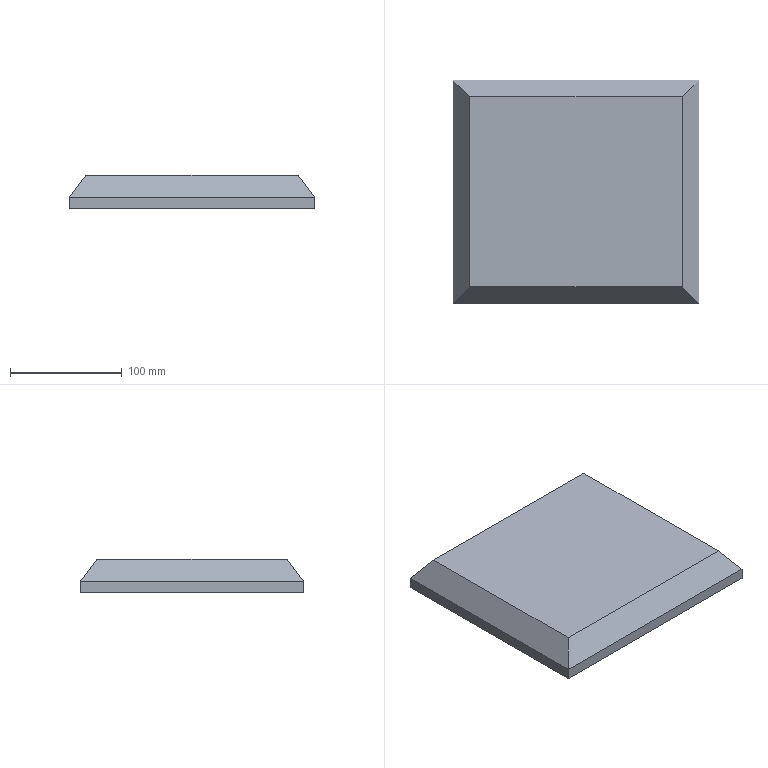Part | SolidWorks | features ICE 1, NetBlend 1 | 1 solid | 10 faces | box 220 x 200 x 30 mm | volume 1200000 mm3 | plane 10
STEP:
#1=CARTESIAN_POINT('',(15.,185.,20.));
#2=VERTEX_POINT('',#1);
#3=CARTESIAN_POINT('',(205.,185.,20.));
#4=VERTEX_POINT('',#3);
#5=CARTESIAN_POINT('',(110.,185.,20.));
#6=DIRECTION('',(1.,0.,0.));
#7=VECTOR('',#6,1000.);
#8=LINE('',#5,#7);
#9=EDGE_CURVE('',#2,#4,#8,.T.);
#10=ORIENTED_EDGE('',*,*,#9,.T.);
#11=CARTESIAN_POINT('',(220.,200.,0.));
#12=VERTEX_POINT('',#11);
#13=CARTESIAN_POINT('',(212.5,192.5,10.));
#14=DIRECTION('',(0.5145,0.5145,-0.686));
#15=VECTOR('',#14,1000.);
#16=LINE('',#13,#15);
#17=EDGE_CURVE('',#4,#12,#16,.T.);
#18=ORIENTED_EDGE('',*,*,#17,.T.);
#19=CARTESIAN_POINT('',(0.,200.,0.));
#20=VERTEX_POINT('',#19);
#21=CARTESIAN_POINT('',(110.,200.,0.));
#22=DIRECTION('',(1.,0.,0.));
#23=VECTOR('',#22,1000.);
#24=LINE('',#21,#23);
#25=EDGE_CURVE('',#20,#12,#24,.T.);
#26=ORIENTED_EDGE('',*,*,#25,.F.);
#27=CARTESIAN_POINT('',(7.5,192.5,10.));
#28=DIRECTION('',(-0.5145,0.5145,-0.686));
#29=VECTOR('',#28,1000.);
#30=LINE('',#27,#29);
#31=EDGE_CURVE('',#2,#20,#30,.T.);
#32=ORIENTED_EDGE('',*,*,#31,.F.);
#33=EDGE_LOOP('',(#10,#18,#26,#32));
#34=FACE_OUTER_BOUND('',#33,.T.);
#35=CARTESIAN_POINT('',(15.,185.,20.));
#36=DIRECTION('',(0.,0.8,0.6));
#37=DIRECTION('',(1.,0.,0.));
#38=AXIS2_PLACEMENT_3D('',#35,#36,#37);
#39=PLANE('',#38);
#40=ADVANCED_FACE('',(#34),#39,.T.);
#41=CARTESIAN_POINT('',(205.,15.,20.));
#42=VERTEX_POINT('',#41);
#43=CARTESIAN_POINT('',(205.,100.,20.));
#44=DIRECTION('',(0.,-1.,0.));
#45=VECTOR('',#44,1000.);
#46=LINE('',#43,#45);
#47=EDGE_CURVE('',#4,#42,#46,.T.);
#48=ORIENTED_EDGE('',*,*,#47,.T.);
#49=CARTESIAN_POINT('',(220.,0.,0.));
#50=VERTEX_POINT('',#49);
#51=CARTESIAN_POINT('',(212.5,7.5,10.));
#52=DIRECTION('',(0.5145,-0.5145,-0.686));
#53=VECTOR('',#52,1000.);
#54=LINE('',#51,#53);
#55=EDGE_CURVE('',#42,#50,#54,.T.);
#56=ORIENTED_EDGE('',*,*,#55,.T.);
#57=CARTESIAN_POINT('',(220.,100.,0.));
#58=DIRECTION('',(0.,-1.,0.));
#59=VECTOR('',#58,1000.);
#60=LINE('',#57,#59);
#61=EDGE_CURVE('',#12,#50,#60,.T.);
#62=ORIENTED_EDGE('',*,*,#61,.F.);
#63=ORIENTED_EDGE('',*,*,#17,.F.);
#64=EDGE_LOOP('',(#48,#56,#62,#63));
#65=FACE_OUTER_BOUND('',#64,.T.);
#66=CARTESIAN_POINT('',(205.,185.,20.));
#67=DIRECTION('',(0.8,0.,0.6));
#68=DIRECTION('',(0.,-1.,0.));
#69=AXIS2_PLACEMENT_3D('',#66,#67,#68);
#70=PLANE('',#69);
#71=ADVANCED_FACE('',(#65),#70,.T.);
#72=CARTESIAN_POINT('',(15.,15.,20.));
#73=VERTEX_POINT('',#72);
#74=CARTESIAN_POINT('',(110.,15.,20.));
#75=DIRECTION('',(-1.,0.,0.));
#76=VECTOR('',#75,1000.);
#77=LINE('',#74,#76);
#78=EDGE_CURVE('',#42,#73,#77,.T.);
#79=ORIENTED_EDGE('',*,*,#78,.T.);
#80=CARTESIAN_POINT('',(0.,0.,0.));
#81=VERTEX_POINT('',#80);
#82=CARTESIAN_POINT('',(7.5,7.5,10.));
#83=DIRECTION('',(-0.5145,-0.5145,-0.686));
#84=VECTOR('',#83,1000.);
#85=LINE('',#82,#84);
#86=EDGE_CURVE('',#73,#81,#85,.T.);
#87=ORIENTED_EDGE('',*,*,#86,.T.);
#88=CARTESIAN_POINT('',(110.,0.,0.));
#89=DIRECTION('',(-1.,0.,0.));
#90=VECTOR('',#89,1000.);
#91=LINE('',#88,#90);
#92=EDGE_CURVE('',#50,#81,#91,.T.);
#93=ORIENTED_EDGE('',*,*,#92,.F.);
#94=ORIENTED_EDGE('',*,*,#55,.F.);
#95=EDGE_LOOP('',(#79,#87,#93,#94));
#96=FACE_OUTER_BOUND('',#95,.T.);
#97=CARTESIAN_POINT('',(205.,15.,20.));
#98=DIRECTION('',(0.,-0.8,0.6));
#99=DIRECTION('',(-1.,0.,0.));
#100=AXIS2_PLACEMENT_3D('',#97,#98,#99);
#101=PLANE('',#100);
#102=ADVANCED_FACE('',(#96),#101,.T.);
#103=CARTESIAN_POINT('',(15.,100.,20.));
#104=DIRECTION('',(0.,1.,0.));
#105=VECTOR('',#104,1000.);
#106=LINE('',#103,#105);
#107=EDGE_CURVE('',#73,#2,#106,.T.);
#108=ORIENTED_EDGE('',*,*,#107,.T.);
#109=ORIENTED_EDGE('',*,*,#31,.T.);
#110=CARTESIAN_POINT('',(0.,100.,0.));
#111=DIRECTION('',(0.,1.,0.));
#112=VECTOR('',#111,1000.);
#113=LINE('',#110,#112);
#114=EDGE_CURVE('',#81,#20,#113,.T.);
#115=ORIENTED_EDGE('',*,*,#114,.F.);
#116=ORIENTED_EDGE('',*,*,#86,.F.);
#117=EDGE_LOOP('',(#108,#109,#115,#116));
#118=FACE_OUTER_BOUND('',#117,.T.);
#119=CARTESIAN_POINT('',(15.,15.,20.));
#120=DIRECTION('',(-0.8,0.,0.6));
#121=DIRECTION('',(0.,1.,0.));
#122=AXIS2_PLACEMENT_3D('',#119,#120,#121);
#123=PLANE('',#122);
#124=ADVANCED_FACE('',(#118),#123,.T.);
#125=ORIENTED_EDGE('',*,*,#107,.F.);
#126=ORIENTED_EDGE('',*,*,#78,.F.);
#127=ORIENTED_EDGE('',*,*,#47,.F.);
#128=ORIENTED_EDGE('',*,*,#9,.F.);
#129=EDGE_LOOP('',(#125,#126,#127,#128));
#130=FACE_OUTER_BOUND('',#129,.T.);
#131=CARTESIAN_POINT('',(0.,0.,20.));
#132=DIRECTION('',(0.,0.,-1.));
#133=DIRECTION('',(-1.,0.,0.));
#134=AXIS2_PLACEMENT_3D('',#131,#132,#133);
#135=PLANE('',#134);
#136=ADVANCED_FACE('',(#130),#135,.F.);
#137=ORIENTED_EDGE('',*,*,#114,.T.);
#138=CARTESIAN_POINT('',(0.,200.,-10.));
#139=VERTEX_POINT('',#138);
#140=CARTESIAN_POINT('',(0.,200.,-10.));
#141=DIRECTION('',(0.,0.,1.));
#142=VECTOR('',#141,1000.);
#143=LINE('',#140,#142);
#144=EDGE_CURVE('',#139,#20,#143,.T.);
#145=ORIENTED_EDGE('',*,*,#144,.F.);
#146=CARTESIAN_POINT('',(0.,0.,-10.));
#147=VERTEX_POINT('',#146);
#148=CARTESIAN_POINT('',(0.,0.,-10.));
#149=DIRECTION('',(0.,1.,0.));
#150=VECTOR('',#149,1000.);
#151=LINE('',#148,#150);
#152=EDGE_CURVE('',#147,#139,#151,.T.);
#153=ORIENTED_EDGE('',*,*,#152,.F.);
#154=CARTESIAN_POINT('',(0.,0.,-10.));
#155=DIRECTION('',(0.,0.,1.));
#156=VECTOR('',#155,1000.);
#157=LINE('',#154,#156);
#158=EDGE_CURVE('',#147,#81,#157,.T.);
#159=ORIENTED_EDGE('',*,*,#158,.T.);
#160=EDGE_LOOP('',(#137,#145,#153,#159));
#161=FACE_OUTER_BOUND('',#160,.T.);
#162=CARTESIAN_POINT('',(0.,0.,-10.));
#163=DIRECTION('',(1.,0.,0.));
#164=DIRECTION('',(0.,0.,-1.));
#165=AXIS2_PLACEMENT_3D('',#162,#163,#164);
#166=PLANE('',#165);
#167=ADVANCED_FACE('',(#161),#166,.F.);
#168=ORIENTED_EDGE('',*,*,#25,.T.);
#169=CARTESIAN_POINT('',(220.,200.,-10.));
#170=VERTEX_POINT('',#169);
#171=CARTESIAN_POINT('',(220.,200.,-10.));
#172=DIRECTION('',(0.,0.,1.));
#173=VECTOR('',#172,1000.);
#174=LINE('',#171,#173);
#175=EDGE_CURVE('',#170,#12,#174,.T.);
#176=ORIENTED_EDGE('',*,*,#175,.F.);
#177=CARTESIAN_POINT('',(0.,200.,-10.));
#178=DIRECTION('',(1.,0.,0.));
#179=VECTOR('',#178,1000.);
#180=LINE('',#177,#179);
#181=EDGE_CURVE('',#139,#170,#180,.T.);
#182=ORIENTED_EDGE('',*,*,#181,.F.);
#183=ORIENTED_EDGE('',*,*,#144,.T.);
#184=EDGE_LOOP('',(#168,#176,#182,#183));
#185=FACE_OUTER_BOUND('',#184,.T.);
#186=CARTESIAN_POINT('',(0.,200.,-10.));
#187=DIRECTION('',(0.,-1.,0.));
#188=DIRECTION('',(0.,0.,-1.));
#189=AXIS2_PLACEMENT_3D('',#186,#187,#188);
#190=PLANE('',#189);
#191=ADVANCED_FACE('',(#185),#190,.F.);
#192=ORIENTED_EDGE('',*,*,#61,.T.);
#193=CARTESIAN_POINT('',(220.,0.,-10.));
#194=VERTEX_POINT('',#193);
#195=CARTESIAN_POINT('',(220.,0.,-10.));
#196=DIRECTION('',(0.,0.,1.));
#197=VECTOR('',#196,1000.);
#198=LINE('',#195,#197);
#199=EDGE_CURVE('',#194,#50,#198,.T.);
#200=ORIENTED_EDGE('',*,*,#199,.F.);
#201=CARTESIAN_POINT('',(220.,200.,-10.));
#202=DIRECTION('',(0.,-1.,0.));
#203=VECTOR('',#202,1000.);
#204=LINE('',#201,#203);
#205=EDGE_CURVE('',#170,#194,#204,.T.);
#206=ORIENTED_EDGE('',*,*,#205,.F.);
#207=ORIENTED_EDGE('',*,*,#175,.T.);
#208=EDGE_LOOP('',(#192,#200,#206,#207));
#209=FACE_OUTER_BOUND('',#208,.T.);
#210=CARTESIAN_POINT('',(220.,200.,-10.));
#211=DIRECTION('',(-1.,0.,0.));
#212=DIRECTION('',(0.,0.,1.));
#213=AXIS2_PLACEMENT_3D('',#210,#211,#212);
#214=PLANE('',#213);
#215=ADVANCED_FACE('',(#209),#214,.F.);
#216=ORIENTED_EDGE('',*,*,#92,.T.);
#217=ORIENTED_EDGE('',*,*,#158,.F.);
#218=CARTESIAN_POINT('',(220.,0.,-10.));
#219=DIRECTION('',(-1.,0.,0.));
#220=VECTOR('',#219,1000.);
#221=LINE('',#218,#220);
#222=EDGE_CURVE('',#194,#147,#221,.T.);
#223=ORIENTED_EDGE('',*,*,#222,.F.);
#224=ORIENTED_EDGE('',*,*,#199,.T.);
#225=EDGE_LOOP('',(#216,#217,#223,#224));
#226=FACE_OUTER_BOUND('',#225,.T.);
#227=CARTESIAN_POINT('',(220.,0.,-10.));
#228=DIRECTION('',(0.,1.,0.));
#229=DIRECTION('',(0.,0.,1.));
#230=AXIS2_PLACEMENT_3D('',#227,#228,#229);
#231=PLANE('',#230);
#232=ADVANCED_FACE('',(#226),#231,.F.);
#233=ORIENTED_EDGE('',*,*,#152,.T.);
#234=ORIENTED_EDGE('',*,*,#181,.T.);
#235=ORIENTED_EDGE('',*,*,#205,.T.);
#236=ORIENTED_EDGE('',*,*,#222,.T.);
#237=EDGE_LOOP('',(#233,#234,#235,#236));
#238=FACE_OUTER_BOUND('',#237,.T.);
#239=CARTESIAN_POINT('',(0.,0.,-10.));
#240=DIRECTION('',(0.,0.,-1.));
#241=DIRECTION('',(-1.,0.,0.));
#242=AXIS2_PLACEMENT_3D('',#239,#240,#241);
#243=PLANE('',#242);
#244=ADVANCED_FACE('',(#238),#243,.T.);
#245=CLOSED_SHELL('',(#40,#71,#102,#124,#136,#167,#191,#215,#232,#244));
#246=MANIFOLD_SOLID_BREP('',#245);
#247=CARTESIAN_POINT('',(0.,0.,0.));
#248=DIRECTION('',(0.,0.,1.));
#249=DIRECTION('',(1.,0.,0.));
#250=AXIS2_PLACEMENT_3D('',#247,#248,#249);
#251=(LENGTH_UNIT()NAMED_UNIT(*)SI_UNIT(.MILLI.,.METRE.));
#252=UNCERTAINTY_MEASURE_WITH_UNIT(LENGTH_MEASURE(0.00001),#251,'','');
#253=(NAMED_UNIT(*)PLANE_ANGLE_UNIT()SI_UNIT($,.RADIAN.));
#254=(NAMED_UNIT(*)SI_UNIT($,.STERADIAN.)SOLID_ANGLE_UNIT());
#255=(GEOMETRIC_REPRESENTATION_CONTEXT(3)GLOBAL_UNCERTAINTY_ASSIGNED_CONTEXT((#252))GLOBAL_UNIT_ASSIGNED_CONTEXT((#251,#253,#254))REPRESENTATION_CONTEXT('',''));
#256=ADVANCED_BREP_SHAPE_REPRESENTATION('',(#246,#250),#255);